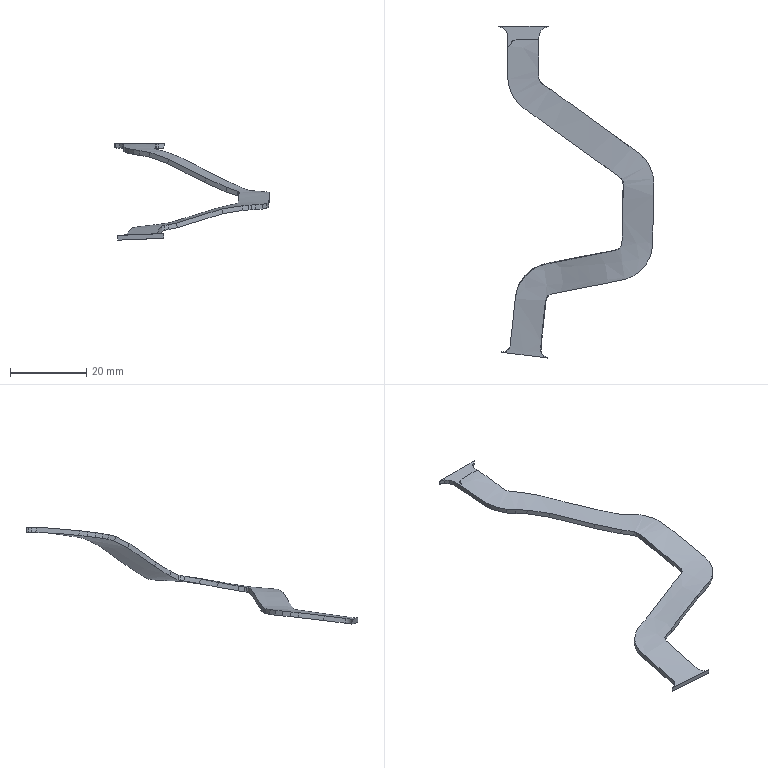Part | STEP file | gslz 2016.10.28-13_id1250_x_t | 1 solid | 74 faces | box 40.597 x 86.839 x 25.215 mm | volume 1239 mm3 | spline 72 | plane 2